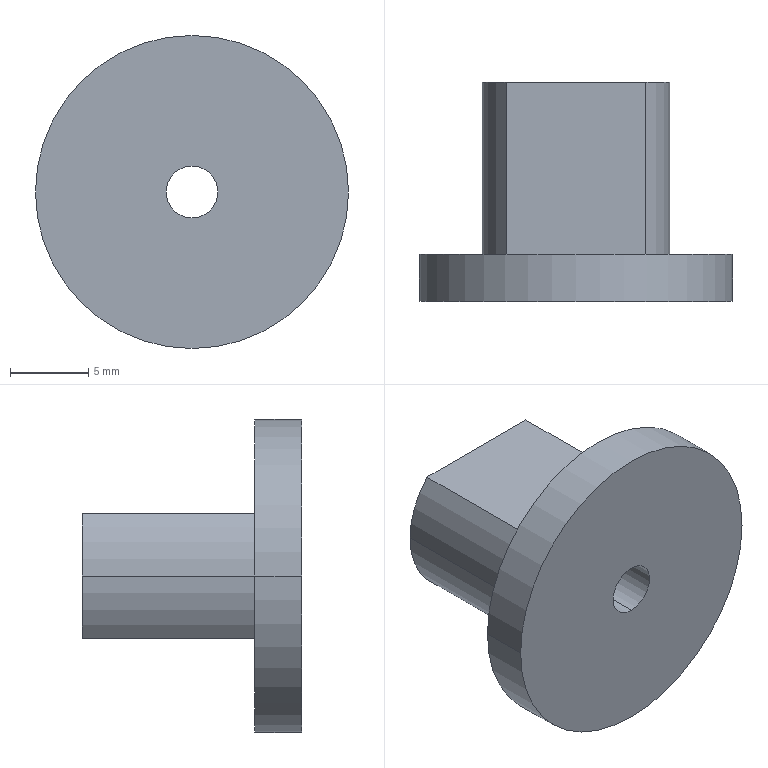Part | STEP file | 0246_212_Nut | 1 solid | 12 faces | box 20 x 14 x 20 mm | volume 1795 mm3 | cylinder 7 | plane 5 | commonest cylinder face diameters 12 x3 3.3 x2 20 x2
STEP:
#1=CARTESIAN_POINT('',(0.,0.,0.));
#2=DIRECTION('',(0.,0.,1.));
#3=DIRECTION('',(1.,0.,0.));
#4=AXIS2_PLACEMENT_3D('',#1,#2,#3);
#5=CARTESIAN_POINT('',(0.,-14.,1.65));
#6=VERTEX_POINT('',#5);
#7=CARTESIAN_POINT('',(0.,0.,1.65));
#8=VERTEX_POINT('',#7);
#9=CARTESIAN_POINT('',(0.,0.,1.65));
#10=DIRECTION('',(0.,1.,0.));
#11=VECTOR('',#10,1.);
#12=LINE('',#9,#11);
#13=CARTESIAN_POINT('',(0.,0.,0.));
#14=DIRECTION('',(0.,1.,0.));
#15=DIRECTION('',(0.,0.,1.));
#16=AXIS2_PLACEMENT_3D('',#13,#14,#15);
#17=CYLINDRICAL_SURFACE('',#16,1.65);
#18=CARTESIAN_POINT('',(6.283,0.));
#19=DIRECTION('',(0.,1.));
#20=VECTOR('',#19,1.);
#21=LINE('',#18,#20);
#22=(GEOMETRIC_REPRESENTATION_CONTEXT(2)PARAMETRIC_REPRESENTATION_CONTEXT()REPRESENTATION_CONTEXT('',''));
#23=DEFINITIONAL_REPRESENTATION('',(#21),#22);
#24=PCURVE('',#17,#23);
#25=CARTESIAN_POINT('',(0.,0.,0.));
#26=DIRECTION('',(0.,1.,0.));
#27=DIRECTION('',(0.,0.,1.));
#28=AXIS2_PLACEMENT_3D('',#25,#26,#27);
#29=CYLINDRICAL_SURFACE('',#28,1.65);
#30=CARTESIAN_POINT('',(0.,0.));
#31=DIRECTION('',(0.,1.));
#32=VECTOR('',#31,1.);
#33=LINE('',#30,#32);
#34=(GEOMETRIC_REPRESENTATION_CONTEXT(2)PARAMETRIC_REPRESENTATION_CONTEXT()REPRESENTATION_CONTEXT('',''));
#35=DEFINITIONAL_REPRESENTATION('',(#33),#34);
#36=PCURVE('',#29,#35);
#37=SURFACE_CURVE('',#12,(#24,#36),.PCURVE_S1.);
#38=EDGE_CURVE('',#6,#8,#37,.T.);
#39=ORIENTED_EDGE('',*,*,#38,.T.);
#40=CARTESIAN_POINT('',(0.,0.,-1.65));
#41=VERTEX_POINT('',#40);
#42=CARTESIAN_POINT('',(0.,0.,0.));
#43=DIRECTION('',(0.,1.,0.));
#44=DIRECTION('',(0.,0.,1.));
#45=AXIS2_PLACEMENT_3D('',#42,#43,#44);
#46=CIRCLE('',#45,1.65);
#47=CARTESIAN_POINT('',(0.,0.));
#48=DIRECTION('',(1.,0.));
#49=VECTOR('',#48,1.);
#50=LINE('',#47,#49);
#51=(GEOMETRIC_REPRESENTATION_CONTEXT(2)PARAMETRIC_REPRESENTATION_CONTEXT()REPRESENTATION_CONTEXT('',''));
#52=DEFINITIONAL_REPRESENTATION('',(#50),#51);
#53=PCURVE('',#17,#52);
#54=CARTESIAN_POINT('',(0.,0.,0.));
#55=DIRECTION('',(0.,1.,0.));
#56=DIRECTION('',(-1.,0.,0.));
#57=AXIS2_PLACEMENT_3D('',#54,#55,#56);
#58=PLANE('',#57);
#59=CARTESIAN_POINT('',(0.,0.));
#60=DIRECTION('',(0.,1.));
#61=AXIS2_PLACEMENT_2D('',#59,#60);
#62=CIRCLE('',#61,1.65);
#63=(GEOMETRIC_REPRESENTATION_CONTEXT(2)PARAMETRIC_REPRESENTATION_CONTEXT()REPRESENTATION_CONTEXT('',''));
#64=DEFINITIONAL_REPRESENTATION('',(#62),#63);
#65=PCURVE('',#58,#64);
#66=SURFACE_CURVE('',#46,(#53,#65),.PCURVE_S1.);
#67=EDGE_CURVE('',#41,#8,#66,.T.);
#68=ORIENTED_EDGE('',*,*,#67,.F.);
#69=CARTESIAN_POINT('',(0.,-14.,-1.65));
#70=VERTEX_POINT('',#69);
#71=CARTESIAN_POINT('',(0.,0.,-1.65));
#72=DIRECTION('',(0.,1.,0.));
#73=VECTOR('',#72,1.);
#74=LINE('',#71,#73);
#75=CARTESIAN_POINT('',(3.142,0.));
#76=DIRECTION('',(0.,1.));
#77=VECTOR('',#76,1.);
#78=LINE('',#75,#77);
#79=(GEOMETRIC_REPRESENTATION_CONTEXT(2)PARAMETRIC_REPRESENTATION_CONTEXT()REPRESENTATION_CONTEXT('',''));
#80=DEFINITIONAL_REPRESENTATION('',(#78),#79);
#81=PCURVE('',#17,#80);
#82=CARTESIAN_POINT('',(3.142,0.));
#83=DIRECTION('',(0.,1.));
#84=VECTOR('',#83,1.);
#85=LINE('',#82,#84);
#86=(GEOMETRIC_REPRESENTATION_CONTEXT(2)PARAMETRIC_REPRESENTATION_CONTEXT()REPRESENTATION_CONTEXT('',''));
#87=DEFINITIONAL_REPRESENTATION('',(#85),#86);
#88=PCURVE('',#29,#87);
#89=SURFACE_CURVE('',#74,(#81,#88),.PCURVE_S1.);
#90=EDGE_CURVE('',#70,#41,#89,.T.);
#91=ORIENTED_EDGE('',*,*,#90,.F.);
#92=CARTESIAN_POINT('',(0.,-14.,0.));
#93=DIRECTION('',(0.,1.,0.));
#94=DIRECTION('',(0.,0.,1.));
#95=AXIS2_PLACEMENT_3D('',#92,#93,#94);
#96=CIRCLE('',#95,1.65);
#97=CARTESIAN_POINT('',(0.,-14.));
#98=DIRECTION('',(1.,0.));
#99=VECTOR('',#98,1.);
#100=LINE('',#97,#99);
#101=(GEOMETRIC_REPRESENTATION_CONTEXT(2)PARAMETRIC_REPRESENTATION_CONTEXT()REPRESENTATION_CONTEXT('',''));
#102=DEFINITIONAL_REPRESENTATION('',(#100),#101);
#103=PCURVE('',#17,#102);
#104=CARTESIAN_POINT('',(10.,-14.,0.));
#105=DIRECTION('',(0.,-1.,0.));
#106=DIRECTION('',(1.,0.,0.));
#107=AXIS2_PLACEMENT_3D('',#104,#105,#106);
#108=PLANE('',#107);
#109=CARTESIAN_POINT('',(-10.,1.65));
#110=CARTESIAN_POINT('',(-7.142,1.65));
#111=CARTESIAN_POINT('',(-8.571,-0.825));
#112=CARTESIAN_POINT('',(-10.,-3.3));
#113=CARTESIAN_POINT('',(-11.429,-0.825));
#114=CARTESIAN_POINT('',(-12.858,1.65));
#115=CARTESIAN_POINT('',(-10.,1.65));
#116=(BOUNDED_CURVE()B_SPLINE_CURVE(2,(#109,#110,#111,#112,#113,#114,#115),.UNSPECIFIED.,.T.,.F.)B_SPLINE_CURVE_WITH_KNOTS((1,2,2,2,2,1),(-2.094,0.,2.094,4.189,6.283,8.378),.UNSPECIFIED.)CURVE()GEOMETRIC_REPRESENTATION_ITEM()RATIONAL_B_SPLINE_CURVE((1.,0.5,1.,0.5,1.,0.5,1.))REPRESENTATION_ITEM(''));
#117=(GEOMETRIC_REPRESENTATION_CONTEXT(2)PARAMETRIC_REPRESENTATION_CONTEXT()REPRESENTATION_CONTEXT('',''));
#118=DEFINITIONAL_REPRESENTATION('',(#116),#117);
#119=PCURVE('',#108,#118);
#120=SURFACE_CURVE('',#96,(#103,#119),.PCURVE_S1.);
#121=EDGE_CURVE('',#70,#6,#120,.T.);
#122=ORIENTED_EDGE('',*,*,#121,.T.);
#123=EDGE_LOOP('',(#39,#68,#91,#122));
#124=FACE_BOUND('',#123,.F.);
#125=ADVANCED_FACE('',(#124),#17,.F.);
#126=CARTESIAN_POINT('',(-10.,-14.,0.));
#127=VERTEX_POINT('',#126);
#128=CARTESIAN_POINT('',(10.,-14.,0.));
#129=VERTEX_POINT('',#128);
#130=CARTESIAN_POINT('',(0.,-14.,0.));
#131=DIRECTION('',(0.,1.,0.));
#132=DIRECTION('',(-1.,0.,0.));
#133=AXIS2_PLACEMENT_3D('',#130,#131,#132);
#134=CIRCLE('',#133,10.);
#135=CARTESIAN_POINT('',(0.,0.,0.));
#136=DIRECTION('',(0.,1.,0.));
#137=DIRECTION('',(-1.,0.,0.));
#138=AXIS2_PLACEMENT_3D('',#135,#136,#137);
#139=CYLINDRICAL_SURFACE('',#138,10.);
#140=CARTESIAN_POINT('',(0.,-14.));
#141=DIRECTION('',(1.,0.));
#142=VECTOR('',#141,1.);
#143=LINE('',#140,#142);
#144=(GEOMETRIC_REPRESENTATION_CONTEXT(2)PARAMETRIC_REPRESENTATION_CONTEXT()REPRESENTATION_CONTEXT('',''));
#145=DEFINITIONAL_REPRESENTATION('',(#143),#144);
#146=PCURVE('',#139,#145);
#147=CARTESIAN_POINT('',(-20.,0.));
#148=CARTESIAN_POINT('',(-20.,17.321));
#149=CARTESIAN_POINT('',(-5.,8.66));
#150=CARTESIAN_POINT('',(10.,0.));
#151=CARTESIAN_POINT('',(-5.,-8.66));
#152=CARTESIAN_POINT('',(-20.,-17.321));
#153=CARTESIAN_POINT('',(-20.,0.));
#154=(BOUNDED_CURVE()B_SPLINE_CURVE(2,(#147,#148,#149,#150,#151,#152,#153),.UNSPECIFIED.,.T.,.F.)B_SPLINE_CURVE_WITH_KNOTS((1,2,2,2,2,1),(-2.094,0.,2.094,4.189,6.283,8.378),.UNSPECIFIED.)CURVE()GEOMETRIC_REPRESENTATION_ITEM()RATIONAL_B_SPLINE_CURVE((1.,0.5,1.,0.5,1.,0.5,1.))REPRESENTATION_ITEM(''));
#155=(GEOMETRIC_REPRESENTATION_CONTEXT(2)PARAMETRIC_REPRESENTATION_CONTEXT()REPRESENTATION_CONTEXT('',''));
#156=DEFINITIONAL_REPRESENTATION('',(#154),#155);
#157=PCURVE('',#108,#156);
#158=SURFACE_CURVE('',#134,(#146,#157),.PCURVE_S1.);
#159=EDGE_CURVE('',#127,#129,#158,.T.);
#160=ORIENTED_EDGE('',*,*,#159,.T.);
#161=CARTESIAN_POINT('',(10.,-11.,0.));
#162=VERTEX_POINT('',#161);
#163=CARTESIAN_POINT('',(10.,0.,0.));
#164=DIRECTION('',(0.,1.,0.));
#165=VECTOR('',#164,1.);
#166=LINE('',#163,#165);
#167=CARTESIAN_POINT('',(3.142,0.));
#168=DIRECTION('',(0.,1.));
#169=VECTOR('',#168,1.);
#170=LINE('',#167,#169);
#171=(GEOMETRIC_REPRESENTATION_CONTEXT(2)PARAMETRIC_REPRESENTATION_CONTEXT()REPRESENTATION_CONTEXT('',''));
#172=DEFINITIONAL_REPRESENTATION('',(#170),#171);
#173=PCURVE('',#139,#172);
#174=CARTESIAN_POINT('',(0.,0.,0.));
#175=DIRECTION('',(0.,1.,0.));
#176=DIRECTION('',(-1.,0.,0.));
#177=AXIS2_PLACEMENT_3D('',#174,#175,#176);
#178=CYLINDRICAL_SURFACE('',#177,10.);
#179=CARTESIAN_POINT('',(3.142,0.));
#180=DIRECTION('',(0.,1.));
#181=VECTOR('',#180,1.);
#182=LINE('',#179,#181);
#183=(GEOMETRIC_REPRESENTATION_CONTEXT(2)PARAMETRIC_REPRESENTATION_CONTEXT()REPRESENTATION_CONTEXT('',''));
#184=DEFINITIONAL_REPRESENTATION('',(#182),#183);
#185=PCURVE('',#178,#184);
#186=SURFACE_CURVE('',#166,(#173,#185),.PCURVE_S1.);
#187=EDGE_CURVE('',#129,#162,#186,.T.);
#188=ORIENTED_EDGE('',*,*,#187,.T.);
#189=CARTESIAN_POINT('',(-10.,-11.,0.));
#190=VERTEX_POINT('',#189);
#191=CARTESIAN_POINT('',(0.,-11.,0.));
#192=DIRECTION('',(0.,1.,0.));
#193=DIRECTION('',(-1.,0.,0.));
#194=AXIS2_PLACEMENT_3D('',#191,#192,#193);
#195=CIRCLE('',#194,10.);
#196=CARTESIAN_POINT('',(0.,-11.));
#197=DIRECTION('',(1.,0.));
#198=VECTOR('',#197,1.);
#199=LINE('',#196,#198);
#200=(GEOMETRIC_REPRESENTATION_CONTEXT(2)PARAMETRIC_REPRESENTATION_CONTEXT()REPRESENTATION_CONTEXT('',''));
#201=DEFINITIONAL_REPRESENTATION('',(#199),#200);
#202=PCURVE('',#139,#201);
#203=CARTESIAN_POINT('',(6.,-11.,0.));
#204=DIRECTION('',(0.,1.,0.));
#205=DIRECTION('',(-1.,0.,0.));
#206=AXIS2_PLACEMENT_3D('',#203,#204,#205);
#207=PLANE('',#206);
#208=CARTESIAN_POINT('',(6.,0.));
#209=DIRECTION('',(1.,0.));
#210=AXIS2_PLACEMENT_2D('',#208,#209);
#211=CIRCLE('',#210,10.);
#212=(GEOMETRIC_REPRESENTATION_CONTEXT(2)PARAMETRIC_REPRESENTATION_CONTEXT()REPRESENTATION_CONTEXT('',''));
#213=DEFINITIONAL_REPRESENTATION('',(#211),#212);
#214=PCURVE('',#207,#213);
#215=SURFACE_CURVE('',#195,(#202,#214),.PCURVE_S1.);
#216=EDGE_CURVE('',#190,#162,#215,.T.);
#217=ORIENTED_EDGE('',*,*,#216,.F.);
#218=CARTESIAN_POINT('',(-10.,0.,0.));
#219=DIRECTION('',(0.,1.,0.));
#220=VECTOR('',#219,1.);
#221=LINE('',#218,#220);
#222=CARTESIAN_POINT('',(0.,0.));
#223=DIRECTION('',(0.,1.));
#224=VECTOR('',#223,1.);
#225=LINE('',#222,#224);
#226=(GEOMETRIC_REPRESENTATION_CONTEXT(2)PARAMETRIC_REPRESENTATION_CONTEXT()REPRESENTATION_CONTEXT('',''));
#227=DEFINITIONAL_REPRESENTATION('',(#225),#226);
#228=PCURVE('',#139,#227);
#229=CARTESIAN_POINT('',(6.283,0.));
#230=DIRECTION('',(0.,1.));
#231=VECTOR('',#230,1.);
#232=LINE('',#229,#231);
#233=(GEOMETRIC_REPRESENTATION_CONTEXT(2)PARAMETRIC_REPRESENTATION_CONTEXT()REPRESENTATION_CONTEXT('',''));
#234=DEFINITIONAL_REPRESENTATION('',(#232),#233);
#235=PCURVE('',#178,#234);
#236=SURFACE_CURVE('',#221,(#228,#235),.PCURVE_S1.);
#237=EDGE_CURVE('',#127,#190,#236,.T.);
#238=ORIENTED_EDGE('',*,*,#237,.F.);
#239=EDGE_LOOP('',(#160,#188,#217,#238));
#240=FACE_BOUND('',#239,.T.);
#241=ADVANCED_FACE('',(#240),#139,.T.);
#242=CARTESIAN_POINT('',(-4.47,-11.,-4.002));
#243=VERTEX_POINT('',#242);
#244=CARTESIAN_POINT('',(-6.,-11.,0.));
#245=VERTEX_POINT('',#244);
#246=CARTESIAN_POINT('',(0.,-11.,0.));
#247=DIRECTION('',(0.,1.,0.));
#248=DIRECTION('',(-1.,0.,0.));
#249=AXIS2_PLACEMENT_3D('',#246,#247,#248);
#250=CIRCLE('',#249,6.);
#251=CARTESIAN_POINT('',(0.,0.,0.));
#252=DIRECTION('',(0.,1.,0.));
#253=DIRECTION('',(-1.,0.,0.));
#254=AXIS2_PLACEMENT_3D('',#251,#252,#253);
#255=CYLINDRICAL_SURFACE('',#254,6.);
#256=CARTESIAN_POINT('',(0.,-11.));
#257=DIRECTION('',(1.,0.));
#258=VECTOR('',#257,1.);
#259=LINE('',#256,#258);
#260=(GEOMETRIC_REPRESENTATION_CONTEXT(2)PARAMETRIC_REPRESENTATION_CONTEXT()REPRESENTATION_CONTEXT('',''));
#261=DEFINITIONAL_REPRESENTATION('',(#259),#260);
#262=PCURVE('',#255,#261);
#263=CARTESIAN_POINT('',(6.,0.));
#264=DIRECTION('',(1.,0.));
#265=AXIS2_PLACEMENT_2D('',#263,#264);
#266=CIRCLE('',#265,6.);
#267=(GEOMETRIC_REPRESENTATION_CONTEXT(2)PARAMETRIC_REPRESENTATION_CONTEXT()REPRESENTATION_CONTEXT('',''));
#268=DEFINITIONAL_REPRESENTATION('',(#266),#267);
#269=PCURVE('',#207,#268);
#270=SURFACE_CURVE('',#250,(#262,#269),.PCURVE_S1.);
#271=EDGE_CURVE('',#243,#245,#270,.T.);
#272=ORIENTED_EDGE('',*,*,#271,.T.);
#273=CARTESIAN_POINT('',(-6.,0.,0.));
#274=VERTEX_POINT('',#273);
#275=CARTESIAN_POINT('',(-6.,0.,0.));
#276=DIRECTION('',(0.,1.,0.));
#277=VECTOR('',#276,1.);
#278=LINE('',#275,#277);
#279=CARTESIAN_POINT('',(6.283,0.));
#280=DIRECTION('',(0.,1.));
#281=VECTOR('',#280,1.);
#282=LINE('',#279,#281);
#283=(GEOMETRIC_REPRESENTATION_CONTEXT(2)PARAMETRIC_REPRESENTATION_CONTEXT()REPRESENTATION_CONTEXT('',''));
#284=DEFINITIONAL_REPRESENTATION('',(#282),#283);
#285=PCURVE('',#255,#284);
#286=CARTESIAN_POINT('',(0.,0.,0.));
#287=DIRECTION('',(0.,1.,0.));
#288=DIRECTION('',(-1.,0.,0.));
#289=AXIS2_PLACEMENT_3D('',#286,#287,#288);
#290=CYLINDRICAL_SURFACE('',#289,6.);
#291=CARTESIAN_POINT('',(0.,0.));
#292=DIRECTION('',(0.,1.));
#293=VECTOR('',#292,1.);
#294=LINE('',#291,#293);
#295=(GEOMETRIC_REPRESENTATION_CONTEXT(2)PARAMETRIC_REPRESENTATION_CONTEXT()REPRESENTATION_CONTEXT('',''));
#296=DEFINITIONAL_REPRESENTATION('',(#294),#295);
#297=PCURVE('',#290,#296);
#298=SURFACE_CURVE('',#278,(#285,#297),.PCURVE_S1.);
#299=EDGE_CURVE('',#245,#274,#298,.T.);
#300=ORIENTED_EDGE('',*,*,#299,.T.);
#301=CARTESIAN_POINT('',(-4.47,0.,-4.002));
#302=VERTEX_POINT('',#301);
#303=CARTESIAN_POINT('',(0.,0.,0.));
#304=DIRECTION('',(0.,1.,0.));
#305=DIRECTION('',(-1.,0.,0.));
#306=AXIS2_PLACEMENT_3D('',#303,#304,#305);
#307=CIRCLE('',#306,6.);
#308=CARTESIAN_POINT('',(0.,0.));
#309=DIRECTION('',(1.,0.));
#310=VECTOR('',#309,1.);
#311=LINE('',#308,#310);
#312=(GEOMETRIC_REPRESENTATION_CONTEXT(2)PARAMETRIC_REPRESENTATION_CONTEXT()REPRESENTATION_CONTEXT('',''));
#313=DEFINITIONAL_REPRESENTATION('',(#311),#312);
#314=PCURVE('',#255,#313);
#315=CARTESIAN_POINT('',(0.,0.));
#316=DIRECTION('',(1.,0.));
#317=AXIS2_PLACEMENT_2D('',#315,#316);
#318=CIRCLE('',#317,6.);
#319=(GEOMETRIC_REPRESENTATION_CONTEXT(2)PARAMETRIC_REPRESENTATION_CONTEXT()REPRESENTATION_CONTEXT('',''));
#320=DEFINITIONAL_REPRESENTATION('',(#318),#319);
#321=PCURVE('',#58,#320);
#322=SURFACE_CURVE('',#307,(#314,#321),.PCURVE_S1.);
#323=EDGE_CURVE('',#302,#274,#322,.T.);
#324=ORIENTED_EDGE('',*,*,#323,.F.);
#325=CARTESIAN_POINT('',(-4.47,-20.16,-4.002));
#326=DIRECTION('',(0.,1.,0.));
#327=VECTOR('',#326,1.);
#328=LINE('',#325,#327);
#329=CARTESIAN_POINT('',(5.553,-20.16));
#330=DIRECTION('',(0.,1.));
#331=VECTOR('',#330,1.);
#332=LINE('',#329,#331);
#333=(GEOMETRIC_REPRESENTATION_CONTEXT(2)PARAMETRIC_REPRESENTATION_CONTEXT()REPRESENTATION_CONTEXT('',''));
#334=DEFINITIONAL_REPRESENTATION('',(#332),#333);
#335=PCURVE('',#255,#334);
#336=CARTESIAN_POINT('',(-4.47,-20.16,-4.002));
#337=DIRECTION('',(0.,0.,1.));
#338=DIRECTION('',(1.,0.,0.));
#339=AXIS2_PLACEMENT_3D('',#336,#337,#338);
#340=PLANE('',#339);
#341=CARTESIAN_POINT('',(0.,0.));
#342=DIRECTION('',(0.,1.));
#343=VECTOR('',#342,1.);
#344=LINE('',#341,#343);
#345=(GEOMETRIC_REPRESENTATION_CONTEXT(2)PARAMETRIC_REPRESENTATION_CONTEXT()REPRESENTATION_CONTEXT('',''));
#346=DEFINITIONAL_REPRESENTATION('',(#344),#345);
#347=PCURVE('',#340,#346);
#348=SURFACE_CURVE('',#328,(#335,#347),.PCURVE_S1.);
#349=EDGE_CURVE('',#243,#302,#348,.T.);
#350=ORIENTED_EDGE('',*,*,#349,.F.);
#351=EDGE_LOOP('',(#272,#300,#324,#350));
#352=FACE_BOUND('',#351,.T.);
#353=ADVANCED_FACE('',(#352),#255,.T.);
#354=CARTESIAN_POINT('',(4.47,-11.,-4.002));
#355=VERTEX_POINT('',#354);
#356=CARTESIAN_POINT('',(4.47,0.,-4.002));
#357=VERTEX_POINT('',#356);
#358=CARTESIAN_POINT('',(4.47,-20.16,-4.002));
#359=DIRECTION('',(0.,1.,0.));
#360=VECTOR('',#359,1.);
#361=LINE('',#358,#360);
#362=CARTESIAN_POINT('',(0.,0.,0.));
#363=DIRECTION('',(0.,1.,0.));
#364=DIRECTION('',(-1.,0.,0.));
#365=AXIS2_PLACEMENT_3D('',#362,#363,#364);
#366=CYLINDRICAL_SURFACE('',#365,6.);
#367=CARTESIAN_POINT('',(3.872,-20.16));
#368=DIRECTION('',(0.,1.));
#369=VECTOR('',#368,1.);
#370=LINE('',#367,#369);
#371=(GEOMETRIC_REPRESENTATION_CONTEXT(2)PARAMETRIC_REPRESENTATION_CONTEXT()REPRESENTATION_CONTEXT('',''));
#372=DEFINITIONAL_REPRESENTATION('',(#370),#371);
#373=PCURVE('',#366,#372);
#374=CARTESIAN_POINT('',(8.94,0.));
#375=DIRECTION('',(0.,1.));
#376=VECTOR('',#375,1.);
#377=LINE('',#374,#376);
#378=(GEOMETRIC_REPRESENTATION_CONTEXT(2)PARAMETRIC_REPRESENTATION_CONTEXT()REPRESENTATION_CONTEXT('',''));
#379=DEFINITIONAL_REPRESENTATION('',(#377),#378);
#380=PCURVE('',#340,#379);
#381=SURFACE_CURVE('',#361,(#373,#380),.PCURVE_S1.);
#382=EDGE_CURVE('',#355,#357,#381,.T.);
#383=ORIENTED_EDGE('',*,*,#382,.T.);
#384=CARTESIAN_POINT('',(4.47,0.,4.002));
#385=VERTEX_POINT('',#384);
#386=CARTESIAN_POINT('',(0.,0.,0.));
#387=DIRECTION('',(0.,1.,0.));
#388=DIRECTION('',(-1.,0.,0.));
#389=AXIS2_PLACEMENT_3D('',#386,#387,#388);
#390=CIRCLE('',#389,6.);
#391=CARTESIAN_POINT('',(0.,0.));
#392=DIRECTION('',(1.,0.));
#393=VECTOR('',#392,1.);
#394=LINE('',#391,#393);
#395=(GEOMETRIC_REPRESENTATION_CONTEXT(2)PARAMETRIC_REPRESENTATION_CONTEXT()REPRESENTATION_CONTEXT('',''));
#396=DEFINITIONAL_REPRESENTATION('',(#394),#395);
#397=PCURVE('',#366,#396);
#398=CARTESIAN_POINT('',(0.,0.));
#399=DIRECTION('',(1.,0.));
#400=AXIS2_PLACEMENT_2D('',#398,#399);
#401=CIRCLE('',#400,6.);
#402=(GEOMETRIC_REPRESENTATION_CONTEXT(2)PARAMETRIC_REPRESENTATION_CONTEXT()REPRESENTATION_CONTEXT('',''));
#403=DEFINITIONAL_REPRESENTATION('',(#401),#402);
#404=PCURVE('',#58,#403);
#405=SURFACE_CURVE('',#390,(#397,#404),.PCURVE_S1.);
#406=EDGE_CURVE('',#385,#357,#405,.T.);
#407=ORIENTED_EDGE('',*,*,#406,.F.);
#408=CARTESIAN_POINT('',(4.47,-11.,4.002));
#409=VERTEX_POINT('',#408);
#410=CARTESIAN_POINT('',(4.47,-20.16,4.002));
#411=DIRECTION('',(0.,1.,0.));
#412=VECTOR('',#411,1.);
#413=LINE('',#410,#412);
#414=CARTESIAN_POINT('',(2.411,-20.16));
#415=DIRECTION('',(0.,1.));
#416=VECTOR('',#415,1.);
#417=LINE('',#414,#416);
#418=(GEOMETRIC_REPRESENTATION_CONTEXT(2)PARAMETRIC_REPRESENTATION_CONTEXT()REPRESENTATION_CONTEXT('',''));
#419=DEFINITIONAL_REPRESENTATION('',(#417),#418);
#420=PCURVE('',#366,#419);
#421=CARTESIAN_POINT('',(-4.47,-20.16,4.002));
#422=DIRECTION('',(0.,0.,-1.));
#423=DIRECTION('',(-1.,0.,0.));
#424=AXIS2_PLACEMENT_3D('',#421,#422,#423);
#425=PLANE('',#424);
#426=CARTESIAN_POINT('',(-8.94,0.));
#427=DIRECTION('',(0.,1.));
#428=VECTOR('',#427,1.);
#429=LINE('',#426,#428);
#430=(GEOMETRIC_REPRESENTATION_CONTEXT(2)PARAMETRIC_REPRESENTATION_CONTEXT()REPRESENTATION_CONTEXT('',''));
#431=DEFINITIONAL_REPRESENTATION('',(#429),#430);
#432=PCURVE('',#425,#431);
#433=SURFACE_CURVE('',#413,(#420,#432),.PCURVE_S1.);
#434=EDGE_CURVE('',#409,#385,#433,.T.);
#435=ORIENTED_EDGE('',*,*,#434,.F.);
#436=CARTESIAN_POINT('',(0.,-11.,0.));
#437=DIRECTION('',(0.,1.,0.));
#438=DIRECTION('',(-1.,0.,0.));
#439=AXIS2_PLACEMENT_3D('',#436,#437,#438);
#440=CIRCLE('',#439,6.);
#441=CARTESIAN_POINT('',(0.,-11.));
#442=DIRECTION('',(1.,0.));
#443=VECTOR('',#442,1.);
#444=LINE('',#441,#443);
#445=(GEOMETRIC_REPRESENTATION_CONTEXT(2)PARAMETRIC_REPRESENTATION_CONTEXT()REPRESENTATION_CONTEXT('',''));
#446=DEFINITIONAL_REPRESENTATION('',(#444),#445);
#447=PCURVE('',#366,#446);
#448=CARTESIAN_POINT('',(6.,0.));
#449=DIRECTION('',(1.,0.));
#450=AXIS2_PLACEMENT_2D('',#448,#449);
#451=CIRCLE('',#450,6.);
#452=(GEOMETRIC_REPRESENTATION_CONTEXT(2)PARAMETRIC_REPRESENTATION_CONTEXT()REPRESENTATION_CONTEXT('',''));
#453=DEFINITIONAL_REPRESENTATION('',(#451),#452);
#454=PCURVE('',#207,#453);
#455=SURFACE_CURVE('',#440,(#447,#454),.PCURVE_S1.);
#456=EDGE_CURVE('',#409,#355,#455,.T.);
#457=ORIENTED_EDGE('',*,*,#456,.T.);
#458=EDGE_LOOP('',(#383,#407,#435,#457));
#459=FACE_BOUND('',#458,.T.);
#460=ADVANCED_FACE('',(#459),#366,.T.);
#461=CARTESIAN_POINT('',(-4.47,0.,-4.002));
#462=DIRECTION('',(1.,0.,0.));
#463=VECTOR('',#462,1.);
#464=LINE('',#461,#463);
#465=CARTESIAN_POINT('',(4.47,-4.002));
#466=DIRECTION('',(-1.,0.));
#467=VECTOR('',#466,1.);
#468=LINE('',#465,#467);
#469=(GEOMETRIC_REPRESENTATION_CONTEXT(2)PARAMETRIC_REPRESENTATION_CONTEXT()REPRESENTATION_CONTEXT('',''));
#470=DEFINITIONAL_REPRESENTATION('',(#468),#469);
#471=PCURVE('',#58,#470);
#472=CARTESIAN_POINT('',(0.,20.16));
#473=DIRECTION('',(1.,0.));
#474=VECTOR('',#473,1.);
#475=LINE('',#472,#474);
#476=(GEOMETRIC_REPRESENTATION_CONTEXT(2)PARAMETRIC_REPRESENTATION_CONTEXT()REPRESENTATION_CONTEXT('',''));
#477=DEFINITIONAL_REPRESENTATION('',(#475),#476);
#478=PCURVE('',#340,#477);
#479=SURFACE_CURVE('',#464,(#471,#478),.PCURVE_S1.);
#480=EDGE_CURVE('',#302,#357,#479,.T.);
#481=ORIENTED_EDGE('',*,*,#480,.F.);
#482=ORIENTED_EDGE('',*,*,#323,.T.);
#483=CARTESIAN_POINT('',(-4.47,0.,4.002));
#484=VERTEX_POINT('',#483);
#485=CARTESIAN_POINT('',(0.,0.,0.));
#486=DIRECTION('',(0.,1.,0.));
#487=DIRECTION('',(-1.,0.,0.));
#488=AXIS2_PLACEMENT_3D('',#485,#486,#487);
#489=CIRCLE('',#488,6.);
#490=CARTESIAN_POINT('',(0.,0.));
#491=DIRECTION('',(1.,0.));
#492=AXIS2_PLACEMENT_2D('',#490,#491);
#493=CIRCLE('',#492,6.);
#494=(GEOMETRIC_REPRESENTATION_CONTEXT(2)PARAMETRIC_REPRESENTATION_CONTEXT()REPRESENTATION_CONTEXT('',''));
#495=DEFINITIONAL_REPRESENTATION('',(#493),#494);
#496=PCURVE('',#58,#495);
#497=CARTESIAN_POINT('',(0.,0.));
#498=DIRECTION('',(1.,0.));
#499=VECTOR('',#498,1.);
#500=LINE('',#497,#499);
#501=(GEOMETRIC_REPRESENTATION_CONTEXT(2)PARAMETRIC_REPRESENTATION_CONTEXT()REPRESENTATION_CONTEXT('',''));
#502=DEFINITIONAL_REPRESENTATION('',(#500),#501);
#503=PCURVE('',#290,#502);
#504=SURFACE_CURVE('',#489,(#496,#503),.PCURVE_S1.);
#505=EDGE_CURVE('',#274,#484,#504,.T.);
#506=ORIENTED_EDGE('',*,*,#505,.T.);
#507=CARTESIAN_POINT('',(-4.47,0.,4.002));
#508=DIRECTION('',(-1.,0.,0.));
#509=VECTOR('',#508,1.);
#510=LINE('',#507,#509);
#511=CARTESIAN_POINT('',(4.47,4.002));
#512=DIRECTION('',(1.,0.));
#513=VECTOR('',#512,1.);
#514=LINE('',#511,#513);
#515=(GEOMETRIC_REPRESENTATION_CONTEXT(2)PARAMETRIC_REPRESENTATION_CONTEXT()REPRESENTATION_CONTEXT('',''));
#516=DEFINITIONAL_REPRESENTATION('',(#514),#515);
#517=PCURVE('',#58,#516);
#518=CARTESIAN_POINT('',(0.,20.16));
#519=DIRECTION('',(1.,0.));
#520=VECTOR('',#519,1.);
#521=LINE('',#518,#520);
#522=(GEOMETRIC_REPRESENTATION_CONTEXT(2)PARAMETRIC_REPRESENTATION_CONTEXT()REPRESENTATION_CONTEXT('',''));
#523=DEFINITIONAL_REPRESENTATION('',(#521),#522);
#524=PCURVE('',#425,#523);
#525=SURFACE_CURVE('',#510,(#517,#524),.PCURVE_S1.);
#526=EDGE_CURVE('',#385,#484,#525,.T.);
#527=ORIENTED_EDGE('',*,*,#526,.F.);
#528=ORIENTED_EDGE('',*,*,#406,.T.);
#529=EDGE_LOOP('',(#481,#482,#506,#527,#528));
#530=FACE_BOUND('',#529,.T.);
#531=CARTESIAN_POINT('',(0.,0.,0.));
#532=DIRECTION('',(0.,1.,0.));
#533=DIRECTION('',(0.,0.,1.));
#534=AXIS2_PLACEMENT_3D('',#531,#532,#533);
#535=CIRCLE('',#534,1.65);
#536=CARTESIAN_POINT('',(0.,0.));
#537=DIRECTION('',(0.,1.));
#538=AXIS2_PLACEMENT_2D('',#536,#537);
#539=CIRCLE('',#538,1.65);
#540=(GEOMETRIC_REPRESENTATION_CONTEXT(2)PARAMETRIC_REPRESENTATION_CONTEXT()REPRESENTATION_CONTEXT('',''));
#541=DEFINITIONAL_REPRESENTATION('',(#539),#540);
#542=PCURVE('',#58,#541);
#543=CARTESIAN_POINT('',(0.,0.));
#544=DIRECTION('',(1.,0.));
#545=VECTOR('',#544,1.);
#546=LINE('',#543,#545);
#547=(GEOMETRIC_REPRESENTATION_CONTEXT(2)PARAMETRIC_REPRESENTATION_CONTEXT()REPRESENTATION_CONTEXT('',''));
#548=DEFINITIONAL_REPRESENTATION('',(#546),#547);
#549=PCURVE('',#29,#548);
#550=SURFACE_CURVE('',#535,(#542,#549),.PCURVE_S1.);
#551=EDGE_CURVE('',#8,#41,#550,.T.);
#552=ORIENTED_EDGE('',*,*,#551,.F.);
#553=ORIENTED_EDGE('',*,*,#67,.F.);
#554=EDGE_LOOP('',(#552,#553));
#555=FACE_BOUND('',#554,.T.);
#556=ADVANCED_FACE('',(#530,#555),#58,.T.);
#557=ORIENTED_EDGE('',*,*,#299,.F.);
#558=CARTESIAN_POINT('',(-4.47,-11.,4.002));
#559=VERTEX_POINT('',#558);
#560=CARTESIAN_POINT('',(0.,-11.,0.));
#561=DIRECTION('',(0.,1.,0.));
#562=DIRECTION('',(-1.,0.,0.));
#563=AXIS2_PLACEMENT_3D('',#560,#561,#562);
#564=CIRCLE('',#563,6.);
#565=CARTESIAN_POINT('',(0.,-11.));
#566=DIRECTION('',(1.,0.));
#567=VECTOR('',#566,1.);
#568=LINE('',#565,#567);
#569=(GEOMETRIC_REPRESENTATION_CONTEXT(2)PARAMETRIC_REPRESENTATION_CONTEXT()REPRESENTATION_CONTEXT('',''));
#570=DEFINITIONAL_REPRESENTATION('',(#568),#569);
#571=PCURVE('',#290,#570);
#572=CARTESIAN_POINT('',(6.,0.));
#573=DIRECTION('',(1.,0.));
#574=AXIS2_PLACEMENT_2D('',#572,#573);
#575=CIRCLE('',#574,6.);
#576=(GEOMETRIC_REPRESENTATION_CONTEXT(2)PARAMETRIC_REPRESENTATION_CONTEXT()REPRESENTATION_CONTEXT('',''));
#577=DEFINITIONAL_REPRESENTATION('',(#575),#576);
#578=PCURVE('',#207,#577);
#579=SURFACE_CURVE('',#564,(#571,#578),.PCURVE_S1.);
#580=EDGE_CURVE('',#245,#559,#579,.T.);
#581=ORIENTED_EDGE('',*,*,#580,.T.);
#582=CARTESIAN_POINT('',(-4.47,-20.16,4.002));
#583=DIRECTION('',(0.,1.,0.));
#584=VECTOR('',#583,1.);
#585=LINE('',#582,#584);
#586=CARTESIAN_POINT('',(0.7303,-20.16));
#587=DIRECTION('',(0.,1.));
#588=VECTOR('',#587,1.);
#589=LINE('',#586,#588);
#590=(GEOMETRIC_REPRESENTATION_CONTEXT(2)PARAMETRIC_REPRESENTATION_CONTEXT()REPRESENTATION_CONTEXT('',''));
#591=DEFINITIONAL_REPRESENTATION('',(#589),#590);
#592=PCURVE('',#290,#591);
#593=CARTESIAN_POINT('',(0.,0.));
#594=DIRECTION('',(0.,1.));
#595=VECTOR('',#594,1.);
#596=LINE('',#593,#595);
#597=(GEOMETRIC_REPRESENTATION_CONTEXT(2)PARAMETRIC_REPRESENTATION_CONTEXT()REPRESENTATION_CONTEXT('',''));
#598=DEFINITIONAL_REPRESENTATION('',(#596),#597);
#599=PCURVE('',#425,#598);
#600=SURFACE_CURVE('',#585,(#592,#599),.PCURVE_S1.);
#601=EDGE_CURVE('',#559,#484,#600,.T.);
#602=ORIENTED_EDGE('',*,*,#601,.T.);
#603=ORIENTED_EDGE('',*,*,#505,.F.);
#604=EDGE_LOOP('',(#557,#581,#602,#603));
#605=FACE_BOUND('',#604,.T.);
#606=ADVANCED_FACE('',(#605),#290,.T.);
#607=ORIENTED_EDGE('',*,*,#216,.T.);
#608=CARTESIAN_POINT('',(0.,-11.,0.));
#609=DIRECTION('',(0.,1.,0.));
#610=DIRECTION('',(-1.,0.,0.));
#611=AXIS2_PLACEMENT_3D('',#608,#609,#610);
#612=CIRCLE('',#611,10.);
#613=CARTESIAN_POINT('',(6.,0.));
#614=DIRECTION('',(1.,0.));
#615=AXIS2_PLACEMENT_2D('',#613,#614);
#616=CIRCLE('',#615,10.);
#617=(GEOMETRIC_REPRESENTATION_CONTEXT(2)PARAMETRIC_REPRESENTATION_CONTEXT()REPRESENTATION_CONTEXT('',''));
#618=DEFINITIONAL_REPRESENTATION('',(#616),#617);
#619=PCURVE('',#207,#618);
#620=CARTESIAN_POINT('',(0.,-11.));
#621=DIRECTION('',(1.,0.));
#622=VECTOR('',#621,1.);
#623=LINE('',#620,#622);
#624=(GEOMETRIC_REPRESENTATION_CONTEXT(2)PARAMETRIC_REPRESENTATION_CONTEXT()REPRESENTATION_CONTEXT('',''));
#625=DEFINITIONAL_REPRESENTATION('',(#623),#624);
#626=PCURVE('',#178,#625);
#627=SURFACE_CURVE('',#612,(#619,#626),.PCURVE_S1.);
#628=EDGE_CURVE('',#162,#190,#627,.T.);
#629=ORIENTED_EDGE('',*,*,#628,.T.);
#630=EDGE_LOOP('',(#607,#629));
#631=FACE_BOUND('',#630,.T.);
#632=ORIENTED_EDGE('',*,*,#456,.F.);
#633=CARTESIAN_POINT('',(-4.47,-11.,4.002));
#634=DIRECTION('',(1.,0.,0.));
#635=VECTOR('',#634,1.);
#636=LINE('',#633,#635);
#637=CARTESIAN_POINT('',(10.47,4.002));
#638=DIRECTION('',(-1.,0.));
#639=VECTOR('',#638,1.);
#640=LINE('',#637,#639);
#641=(GEOMETRIC_REPRESENTATION_CONTEXT(2)PARAMETRIC_REPRESENTATION_CONTEXT()REPRESENTATION_CONTEXT('',''));
#642=DEFINITIONAL_REPRESENTATION('',(#640),#641);
#643=PCURVE('',#207,#642);
#644=CARTESIAN_POINT('',(0.,9.16));
#645=DIRECTION('',(-1.,0.));
#646=VECTOR('',#645,1.);
#647=LINE('',#644,#646);
#648=(GEOMETRIC_REPRESENTATION_CONTEXT(2)PARAMETRIC_REPRESENTATION_CONTEXT()REPRESENTATION_CONTEXT('',''));
#649=DEFINITIONAL_REPRESENTATION('',(#647),#648);
#650=PCURVE('',#425,#649);
#651=SURFACE_CURVE('',#636,(#643,#650),.PCURVE_S1.);
#652=EDGE_CURVE('',#559,#409,#651,.T.);
#653=ORIENTED_EDGE('',*,*,#652,.F.);
#654=ORIENTED_EDGE('',*,*,#580,.F.);
#655=ORIENTED_EDGE('',*,*,#271,.F.);
#656=CARTESIAN_POINT('',(-4.47,-11.,-4.002));
#657=DIRECTION('',(-1.,0.,0.));
#658=VECTOR('',#657,1.);
#659=LINE('',#656,#658);
#660=CARTESIAN_POINT('',(10.47,-4.002));
#661=DIRECTION('',(1.,0.));
#662=VECTOR('',#661,1.);
#663=LINE('',#660,#662);
#664=(GEOMETRIC_REPRESENTATION_CONTEXT(2)PARAMETRIC_REPRESENTATION_CONTEXT()REPRESENTATION_CONTEXT('',''));
#665=DEFINITIONAL_REPRESENTATION('',(#663),#664);
#666=PCURVE('',#207,#665);
#667=CARTESIAN_POINT('',(0.,9.16));
#668=DIRECTION('',(-1.,0.));
#669=VECTOR('',#668,1.);
#670=LINE('',#667,#669);
#671=(GEOMETRIC_REPRESENTATION_CONTEXT(2)PARAMETRIC_REPRESENTATION_CONTEXT()REPRESENTATION_CONTEXT('',''));
#672=DEFINITIONAL_REPRESENTATION('',(#670),#671);
#673=PCURVE('',#340,#672);
#674=SURFACE_CURVE('',#659,(#666,#673),.PCURVE_S1.);
#675=EDGE_CURVE('',#355,#243,#674,.T.);
#676=ORIENTED_EDGE('',*,*,#675,.F.);
#677=EDGE_LOOP('',(#632,#653,#654,#655,#676));
#678=FACE_BOUND('',#677,.T.);
#679=ADVANCED_FACE('',(#631,#678),#207,.T.);
#680=ORIENTED_EDGE('',*,*,#187,.F.);
#681=CARTESIAN_POINT('',(0.,-14.,0.));
#682=DIRECTION('',(0.,1.,0.));
#683=DIRECTION('',(-1.,0.,0.));
#684=AXIS2_PLACEMENT_3D('',#681,#682,#683);
#685=CIRCLE('',#684,10.);
#686=CARTESIAN_POINT('',(0.,-14.));
#687=DIRECTION('',(1.,0.));
#688=VECTOR('',#687,1.);
#689=LINE('',#686,#688);
#690=(GEOMETRIC_REPRESENTATION_CONTEXT(2)PARAMETRIC_REPRESENTATION_CONTEXT()REPRESENTATION_CONTEXT('',''));
#691=DEFINITIONAL_REPRESENTATION('',(#689),#690);
#692=PCURVE('',#178,#691);
#693=CARTESIAN_POINT('',(-20.,0.));
#694=CARTESIAN_POINT('',(-20.,17.321));
#695=CARTESIAN_POINT('',(-5.,8.66));
#696=CARTESIAN_POINT('',(10.,0.));
#697=CARTESIAN_POINT('',(-5.,-8.66));
#698=CARTESIAN_POINT('',(-20.,-17.321));
#699=CARTESIAN_POINT('',(-20.,0.));
#700=(BOUNDED_CURVE()B_SPLINE_CURVE(2,(#693,#694,#695,#696,#697,#698,#699),.UNSPECIFIED.,.T.,.F.)B_SPLINE_CURVE_WITH_KNOTS((1,2,2,2,2,1),(-2.094,0.,2.094,4.189,6.283,8.378),.UNSPECIFIED.)CURVE()GEOMETRIC_REPRESENTATION_ITEM()RATIONAL_B_SPLINE_CURVE((1.,0.5,1.,0.5,1.,0.5,1.))REPRESENTATION_ITEM(''));
#701=(GEOMETRIC_REPRESENTATION_CONTEXT(2)PARAMETRIC_REPRESENTATION_CONTEXT()REPRESENTATION_CONTEXT('',''));
#702=DEFINITIONAL_REPRESENTATION('',(#700),#701);
#703=PCURVE('',#108,#702);
#704=SURFACE_CURVE('',#685,(#692,#703),.PCURVE_S1.);
#705=EDGE_CURVE('',#129,#127,#704,.T.);
#706=ORIENTED_EDGE('',*,*,#705,.T.);
#707=ORIENTED_EDGE('',*,*,#237,.T.);
#708=ORIENTED_EDGE('',*,*,#628,.F.);
#709=EDGE_LOOP('',(#680,#706,#707,#708));
#710=FACE_BOUND('',#709,.T.);
#711=ADVANCED_FACE('',(#710),#178,.T.);
#712=CARTESIAN_POINT('',(0.,-14.,0.));
#713=DIRECTION('',(0.,1.,0.));
#714=DIRECTION('',(0.,0.,1.));
#715=AXIS2_PLACEMENT_3D('',#712,#713,#714);
#716=CIRCLE('',#715,1.65);
#717=CARTESIAN_POINT('',(-10.,1.65));
#718=CARTESIAN_POINT('',(-7.142,1.65));
#719=CARTESIAN_POINT('',(-8.571,-0.825));
#720=CARTESIAN_POINT('',(-10.,-3.3));
#721=CARTESIAN_POINT('',(-11.429,-0.825));
#722=CARTESIAN_POINT('',(-12.858,1.65));
#723=CARTESIAN_POINT('',(-10.,1.65));
#724=(BOUNDED_CURVE()B_SPLINE_CURVE(2,(#717,#718,#719,#720,#721,#722,#723),.UNSPECIFIED.,.T.,.F.)B_SPLINE_CURVE_WITH_KNOTS((1,2,2,2,2,1),(-2.094,0.,2.094,4.189,6.283,8.378),.UNSPECIFIED.)CURVE()GEOMETRIC_REPRESENTATION_ITEM()RATIONAL_B_SPLINE_CURVE((1.,0.5,1.,0.5,1.,0.5,1.))REPRESENTATION_ITEM(''));
#725=(GEOMETRIC_REPRESENTATION_CONTEXT(2)PARAMETRIC_REPRESENTATION_CONTEXT()REPRESENTATION_CONTEXT('',''));
#726=DEFINITIONAL_REPRESENTATION('',(#724),#725);
#727=PCURVE('',#108,#726);
#728=CARTESIAN_POINT('',(0.,-14.));
#729=DIRECTION('',(1.,0.));
#730=VECTOR('',#729,1.);
#731=LINE('',#728,#730);
#732=(GEOMETRIC_REPRESENTATION_CONTEXT(2)PARAMETRIC_REPRESENTATION_CONTEXT()REPRESENTATION_CONTEXT('',''));
#733=DEFINITIONAL_REPRESENTATION('',(#731),#732);
#734=PCURVE('',#29,#733);
#735=SURFACE_CURVE('',#716,(#727,#734),.PCURVE_S1.);
#736=EDGE_CURVE('',#6,#70,#735,.T.);
#737=ORIENTED_EDGE('',*,*,#736,.T.);
#738=ORIENTED_EDGE('',*,*,#121,.T.);
#739=EDGE_LOOP('',(#737,#738));
#740=FACE_BOUND('',#739,.T.);
#741=ORIENTED_EDGE('',*,*,#159,.F.);
#742=ORIENTED_EDGE('',*,*,#705,.F.);
#743=EDGE_LOOP('',(#741,#742));
#744=FACE_BOUND('',#743,.T.);
#745=ADVANCED_FACE('',(#740,#744),#108,.T.);
#746=ORIENTED_EDGE('',*,*,#551,.F.);
#747=ORIENTED_EDGE('',*,*,#38,.F.);
#748=ORIENTED_EDGE('',*,*,#736,.T.);
#749=ORIENTED_EDGE('',*,*,#90,.T.);
#750=EDGE_LOOP('',(#746,#747,#748,#749));
#751=FACE_BOUND('',#750,.F.);
#752=ADVANCED_FACE('',(#751),#29,.F.);
#753=ORIENTED_EDGE('',*,*,#652,.T.);
#754=ORIENTED_EDGE('',*,*,#434,.T.);
#755=ORIENTED_EDGE('',*,*,#526,.T.);
#756=ORIENTED_EDGE('',*,*,#601,.F.);
#757=EDGE_LOOP('',(#753,#754,#755,#756));
#758=FACE_BOUND('',#757,.T.);
#759=ADVANCED_FACE('',(#758),#425,.F.);
#760=ORIENTED_EDGE('',*,*,#675,.T.);
#761=ORIENTED_EDGE('',*,*,#349,.T.);
#762=ORIENTED_EDGE('',*,*,#480,.T.);
#763=ORIENTED_EDGE('',*,*,#382,.F.);
#764=EDGE_LOOP('',(#760,#761,#762,#763));
#765=FACE_BOUND('',#764,.T.);
#766=ADVANCED_FACE('',(#765),#340,.F.);
#767=CLOSED_SHELL('',(#125,#241,#353,#460,#556,#606,#679,#711,#745,#752,#759,#766));
#768=MANIFOLD_SOLID_BREP('',#767);
#769=(LENGTH_UNIT()NAMED_UNIT(*)SI_UNIT(.MILLI.,.METRE.));
#770=UNCERTAINTY_MEASURE_WITH_UNIT(LENGTH_MEASURE(0.0000001),#769,'','');
#771=(NAMED_UNIT(*)PLANE_ANGLE_UNIT()SI_UNIT($,.RADIAN.));
#772=(NAMED_UNIT(*)SI_UNIT($,.STERADIAN.)SOLID_ANGLE_UNIT());
#773=(GEOMETRIC_REPRESENTATION_CONTEXT(3)GLOBAL_UNCERTAINTY_ASSIGNED_CONTEXT((#770))GLOBAL_UNIT_ASSIGNED_CONTEXT((#769,#771,#772))REPRESENTATION_CONTEXT('',''));
#774=ADVANCED_BREP_SHAPE_REPRESENTATION('',(#4,#768),#773);